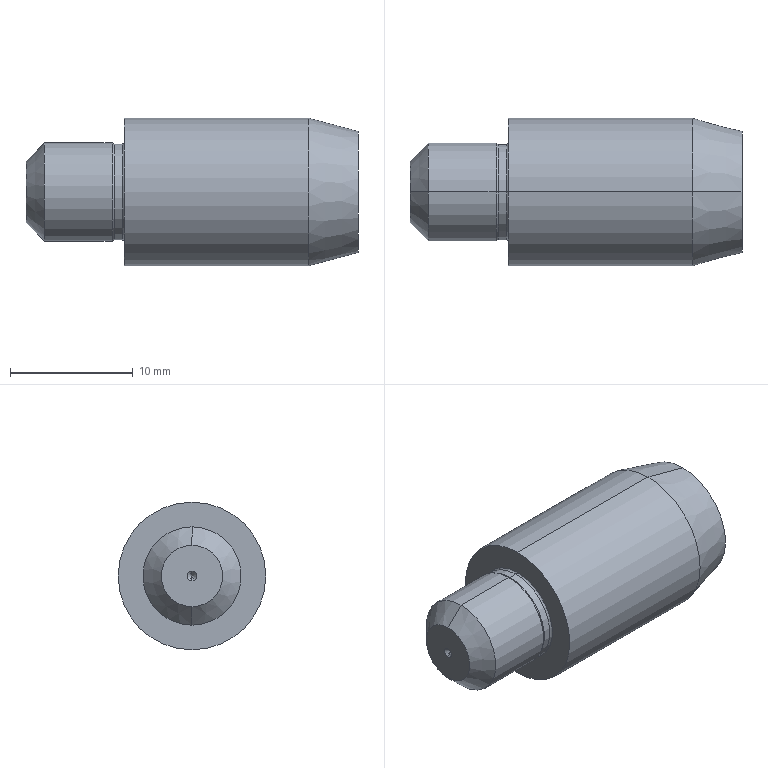Part | STEP file | FPBA8_P12_L9_B15_FPBA8-P12-L8-B15 | 1 solid | 21 faces | box 27 x 12 x 12 mm | volume 2448 mm3 | cone 8 | cylinder 6 | torus 4 | plane 3 | commonest cylinder face diameters 7.8 x2 8 x2 12 x2
STEP:
#1=CARTESIAN_POINT('',(0.,0.,0.));
#2=DIRECTION('',(0.,0.,1.));
#3=DIRECTION('',(1.,0.,0.));
#4=AXIS2_PLACEMENT_3D('',#1,#2,#3);
#5=CARTESIAN_POINT('',(19.,0.,-0.4));
#6=VERTEX_POINT('',#5);
#7=CARTESIAN_POINT('',(19.,0.,0.4));
#8=VERTEX_POINT('',#7);
#9=CARTESIAN_POINT('',(19.,0.,0.));
#10=DIRECTION('',(-1.,0.,0.));
#11=DIRECTION('',(0.,0.,1.));
#12=AXIS2_PLACEMENT_3D('',#9,#10,#11);
#13=CIRCLE('',#12,0.4);
#14=CARTESIAN_POINT('',(1018.6,0.,0.));
#15=DIRECTION('',(1.,0.,0.));
#16=DIRECTION('',(0.,0.,-1.));
#17=AXIS2_PLACEMENT_3D('',#14,#15,#16);
#18=CONICAL_SURFACE('',#17,1000.,0.7854);
#19=CARTESIAN_POINT('',(9.425,-999.6));
#20=DIRECTION('',(-1.,0.));
#21=VECTOR('',#20,1.);
#22=LINE('',#19,#21);
#23=(GEOMETRIC_REPRESENTATION_CONTEXT(2)PARAMETRIC_REPRESENTATION_CONTEXT()REPRESENTATION_CONTEXT('',''));
#24=DEFINITIONAL_REPRESENTATION('',(#22),#23);
#25=PCURVE('',#18,#24);
#26=CARTESIAN_POINT('',(19.,4.928,0.));
#27=DIRECTION('',(-1.,0.,0.));
#28=DIRECTION('',(0.,0.,1.));
#29=AXIS2_PLACEMENT_3D('',#26,#27,#28);
#30=PLANE('',#29);
#31=CARTESIAN_POINT('',(0.,-4.928));
#32=DIRECTION('',(1.,0.));
#33=AXIS2_PLACEMENT_2D('',#31,#32);
#34=CIRCLE('',#33,0.4);
#35=(GEOMETRIC_REPRESENTATION_CONTEXT(2)PARAMETRIC_REPRESENTATION_CONTEXT()REPRESENTATION_CONTEXT('',''));
#36=DEFINITIONAL_REPRESENTATION('',(#34),#35);
#37=PCURVE('',#30,#36);
#38=SURFACE_CURVE('',#13,(#25,#37),.PCURVE_S1.);
#39=EDGE_CURVE('',#6,#8,#38,.T.);
#40=ORIENTED_EDGE('',*,*,#39,.T.);
#41=CARTESIAN_POINT('',(18.6,0.,0.));
#42=VERTEX_POINT('',#41);
#43=CARTESIAN_POINT('',(18.6,0.,0.));
#44=DIRECTION('',(0.7071,0.,0.7071));
#45=VECTOR('',#44,1.);
#46=LINE('',#43,#45);
#47=CARTESIAN_POINT('',(3.142,-1000.));
#48=CARTESIAN_POINT('',(3.142,-999.994));
#49=CARTESIAN_POINT('',(3.142,-999.982));
#50=CARTESIAN_POINT('',(3.142,-999.964));
#51=CARTESIAN_POINT('',(3.142,-999.945));
#52=CARTESIAN_POINT('',(3.142,-999.927));
#53=CARTESIAN_POINT('',(3.142,-999.909));
#54=CARTESIAN_POINT('',(3.142,-999.891));
#55=CARTESIAN_POINT('',(3.142,-999.873));
#56=CARTESIAN_POINT('',(3.142,-999.855));
#57=CARTESIAN_POINT('',(3.142,-999.836));
#58=CARTESIAN_POINT('',(3.142,-999.818));
#59=CARTESIAN_POINT('',(3.142,-999.8));
#60=CARTESIAN_POINT('',(3.142,-999.782));
#61=CARTESIAN_POINT('',(3.142,-999.764));
#62=CARTESIAN_POINT('',(3.142,-999.745));
#63=CARTESIAN_POINT('',(3.142,-999.727));
#64=CARTESIAN_POINT('',(3.142,-999.709));
#65=CARTESIAN_POINT('',(3.142,-999.691));
#66=CARTESIAN_POINT('',(3.142,-999.673));
#67=CARTESIAN_POINT('',(3.142,-999.655));
#68=CARTESIAN_POINT('',(3.142,-999.636));
#69=CARTESIAN_POINT('',(3.142,-999.618));
#70=CARTESIAN_POINT('',(3.142,-999.606));
#71=CARTESIAN_POINT('',(3.142,-999.6));
#72=B_SPLINE_CURVE_WITH_KNOTS('',3,(#47,#48,#49,#50,#51,#52,#53,#54,#55,#56,#57,#58,#59,#60,#61,#62,#63,#64,#65,#66,#67,#68,#69,#70,#71),.UNSPECIFIED.,.F.,.F.,(4,1,1,1,1,1,1,1,1,1,1,1,1,1,1,1,1,1,1,1,1,1,4),(0.,0.02571,0.05143,0.07714,0.1029,0.1286,0.1543,0.18,0.2057,0.2314,0.2571,0.2828,0.3086,0.3343,0.36,0.3857,0.4114,0.4371,0.4628,0.4885,0.5143,0.54,0.5657),.QUASI_UNIFORM_KNOTS.);
#73=(GEOMETRIC_REPRESENTATION_CONTEXT(2)PARAMETRIC_REPRESENTATION_CONTEXT()REPRESENTATION_CONTEXT('',''));
#74=DEFINITIONAL_REPRESENTATION('',(#72),#73);
#75=PCURVE('',#18,#74);
#76=CARTESIAN_POINT('',(1018.6,0.,0.));
#77=DIRECTION('',(1.,0.,0.));
#78=DIRECTION('',(0.,0.,-1.));
#79=AXIS2_PLACEMENT_3D('',#76,#77,#78);
#80=CONICAL_SURFACE('',#79,1000.,0.7854);
#81=CARTESIAN_POINT('',(3.142,-1000.));
#82=CARTESIAN_POINT('',(3.142,-999.994));
#83=CARTESIAN_POINT('',(3.142,-999.982));
#84=CARTESIAN_POINT('',(3.142,-999.964));
#85=CARTESIAN_POINT('',(3.142,-999.945));
#86=CARTESIAN_POINT('',(3.142,-999.927));
#87=CARTESIAN_POINT('',(3.142,-999.909));
#88=CARTESIAN_POINT('',(3.142,-999.891));
#89=CARTESIAN_POINT('',(3.142,-999.873));
#90=CARTESIAN_POINT('',(3.142,-999.855));
#91=CARTESIAN_POINT('',(3.142,-999.836));
#92=CARTESIAN_POINT('',(3.142,-999.818));
#93=CARTESIAN_POINT('',(3.142,-999.8));
#94=CARTESIAN_POINT('',(3.142,-999.782));
#95=CARTESIAN_POINT('',(3.142,-999.764));
#96=CARTESIAN_POINT('',(3.142,-999.745));
#97=CARTESIAN_POINT('',(3.142,-999.727));
#98=CARTESIAN_POINT('',(3.142,-999.709));
#99=CARTESIAN_POINT('',(3.142,-999.691));
#100=CARTESIAN_POINT('',(3.142,-999.673));
#101=CARTESIAN_POINT('',(3.142,-999.655));
#102=CARTESIAN_POINT('',(3.142,-999.636));
#103=CARTESIAN_POINT('',(3.142,-999.618));
#104=CARTESIAN_POINT('',(3.142,-999.606));
#105=CARTESIAN_POINT('',(3.142,-999.6));
#106=B_SPLINE_CURVE_WITH_KNOTS('',3,(#81,#82,#83,#84,#85,#86,#87,#88,#89,#90,#91,#92,#93,#94,#95,#96,#97,#98,#99,#100,#101,#102,#103,#104,#105),.UNSPECIFIED.,.F.,.F.,(4,1,1,1,1,1,1,1,1,1,1,1,1,1,1,1,1,1,1,1,1,1,4),(0.,0.02571,0.05143,0.07714,0.1029,0.1286,0.1543,0.18,0.2057,0.2314,0.2571,0.2828,0.3086,0.3343,0.36,0.3857,0.4114,0.4371,0.4628,0.4885,0.5143,0.54,0.5657),.QUASI_UNIFORM_KNOTS.);
#107=(GEOMETRIC_REPRESENTATION_CONTEXT(2)PARAMETRIC_REPRESENTATION_CONTEXT()REPRESENTATION_CONTEXT('',''));
#108=DEFINITIONAL_REPRESENTATION('',(#106),#107);
#109=PCURVE('',#80,#108);
#110=SURFACE_CURVE('',#46,(#75,#109),.PCURVE_S1.);
#111=EDGE_CURVE('',#42,#8,#110,.T.);
#112=ORIENTED_EDGE('',*,*,#111,.F.);
#113=CARTESIAN_POINT('',(18.6,0.,0.));
#114=DIRECTION('',(0.7071,0.,-0.7071));
#115=VECTOR('',#114,1.);
#116=LINE('',#113,#115);
#117=CARTESIAN_POINT('',(6.283,-1000.));
#118=DIRECTION('',(0.,1.));
#119=VECTOR('',#118,1.);
#120=LINE('',#117,#119);
#121=(GEOMETRIC_REPRESENTATION_CONTEXT(2)PARAMETRIC_REPRESENTATION_CONTEXT()REPRESENTATION_CONTEXT('',''));
#122=DEFINITIONAL_REPRESENTATION('',(#120),#121);
#123=PCURVE('',#18,#122);
#124=CARTESIAN_POINT('',(0.,-1000.));
#125=DIRECTION('',(0.,1.));
#126=VECTOR('',#125,1.);
#127=LINE('',#124,#126);
#128=(GEOMETRIC_REPRESENTATION_CONTEXT(2)PARAMETRIC_REPRESENTATION_CONTEXT()REPRESENTATION_CONTEXT('',''));
#129=DEFINITIONAL_REPRESENTATION('',(#127),#128);
#130=PCURVE('',#80,#129);
#131=SURFACE_CURVE('',#116,(#123,#130),.PCURVE_S1.);
#132=EDGE_CURVE('',#42,#6,#131,.T.);
#133=ORIENTED_EDGE('',*,*,#132,.T.);
#134=EDGE_LOOP('',(#40,#112,#133));
#135=FACE_BOUND('',#134,.F.);
#136=ADVANCED_FACE('',(#135),#18,.F.);
#137=CARTESIAN_POINT('',(19.,0.,4.928));
#138=VERTEX_POINT('',#137);
#139=CARTESIAN_POINT('',(19.,0.,-4.928));
#140=VERTEX_POINT('',#139);
#141=CARTESIAN_POINT('',(19.,0.,0.));
#142=DIRECTION('',(-1.,0.,0.));
#143=DIRECTION('',(0.,0.,1.));
#144=AXIS2_PLACEMENT_3D('',#141,#142,#143);
#145=CIRCLE('',#144,4.928);
#146=CARTESIAN_POINT('',(19.,0.,0.));
#147=DIRECTION('',(-1.,0.,0.));
#148=DIRECTION('',(0.,0.,1.));
#149=AXIS2_PLACEMENT_3D('',#146,#147,#148);
#150=CONICAL_SURFACE('',#149,4.928,0.2618);
#151=CARTESIAN_POINT('',(0.,0.));
#152=DIRECTION('',(1.,0.));
#153=VECTOR('',#152,1.);
#154=LINE('',#151,#153);
#155=(GEOMETRIC_REPRESENTATION_CONTEXT(2)PARAMETRIC_REPRESENTATION_CONTEXT()REPRESENTATION_CONTEXT('',''));
#156=DEFINITIONAL_REPRESENTATION('',(#154),#155);
#157=PCURVE('',#150,#156);
#158=CARTESIAN_POINT('',(0.,-4.928));
#159=DIRECTION('',(1.,0.));
#160=AXIS2_PLACEMENT_2D('',#158,#159);
#161=CIRCLE('',#160,4.928);
#162=(GEOMETRIC_REPRESENTATION_CONTEXT(2)PARAMETRIC_REPRESENTATION_CONTEXT()REPRESENTATION_CONTEXT('',''));
#163=DEFINITIONAL_REPRESENTATION('',(#161),#162);
#164=PCURVE('',#30,#163);
#165=SURFACE_CURVE('',#145,(#157,#164),.PCURVE_S1.);
#166=EDGE_CURVE('',#138,#140,#165,.T.);
#167=ORIENTED_EDGE('',*,*,#166,.T.);
#168=CARTESIAN_POINT('',(15.,0.,-6.));
#169=VERTEX_POINT('',#168);
#170=CARTESIAN_POINT('',(19.,0.,-4.928));
#171=DIRECTION('',(-0.9659,0.,-0.2588));
#172=VECTOR('',#171,1.);
#173=LINE('',#170,#172);
#174=CARTESIAN_POINT('',(3.142,0.));
#175=DIRECTION('',(0.,1.));
#176=VECTOR('',#175,1.);
#177=LINE('',#174,#176);
#178=(GEOMETRIC_REPRESENTATION_CONTEXT(2)PARAMETRIC_REPRESENTATION_CONTEXT()REPRESENTATION_CONTEXT('',''));
#179=DEFINITIONAL_REPRESENTATION('',(#177),#178);
#180=PCURVE('',#150,#179);
#181=CARTESIAN_POINT('',(19.,0.,0.));
#182=DIRECTION('',(-1.,0.,0.));
#183=DIRECTION('',(0.,0.,1.));
#184=AXIS2_PLACEMENT_3D('',#181,#182,#183);
#185=CONICAL_SURFACE('',#184,4.928,0.2618);
#186=CARTESIAN_POINT('',(3.142,0.));
#187=DIRECTION('',(0.,1.));
#188=VECTOR('',#187,1.);
#189=LINE('',#186,#188);
#190=(GEOMETRIC_REPRESENTATION_CONTEXT(2)PARAMETRIC_REPRESENTATION_CONTEXT()REPRESENTATION_CONTEXT('',''));
#191=DEFINITIONAL_REPRESENTATION('',(#189),#190);
#192=PCURVE('',#185,#191);
#193=SURFACE_CURVE('',#173,(#180,#192),.PCURVE_S1.);
#194=EDGE_CURVE('',#140,#169,#193,.T.);
#195=ORIENTED_EDGE('',*,*,#194,.T.);
#196=CARTESIAN_POINT('',(15.,0.,6.));
#197=VERTEX_POINT('',#196);
#198=CARTESIAN_POINT('',(15.,0.,0.));
#199=DIRECTION('',(-1.,0.,0.));
#200=DIRECTION('',(0.,0.,1.));
#201=AXIS2_PLACEMENT_3D('',#198,#199,#200);
#202=CIRCLE('',#201,6.);
#203=CARTESIAN_POINT('',(0.,4.));
#204=DIRECTION('',(1.,0.));
#205=VECTOR('',#204,1.);
#206=LINE('',#203,#205);
#207=(GEOMETRIC_REPRESENTATION_CONTEXT(2)PARAMETRIC_REPRESENTATION_CONTEXT()REPRESENTATION_CONTEXT('',''));
#208=DEFINITIONAL_REPRESENTATION('',(#206),#207);
#209=PCURVE('',#150,#208);
#210=CARTESIAN_POINT('',(18.6,0.,0.));
#211=DIRECTION('',(-1.,0.,0.));
#212=DIRECTION('',(0.,0.,1.));
#213=AXIS2_PLACEMENT_3D('',#210,#211,#212);
#214=CYLINDRICAL_SURFACE('',#213,6.);
#215=CARTESIAN_POINT('',(0.,3.6));
#216=DIRECTION('',(1.,0.));
#217=VECTOR('',#216,1.);
#218=LINE('',#215,#217);
#219=(GEOMETRIC_REPRESENTATION_CONTEXT(2)PARAMETRIC_REPRESENTATION_CONTEXT()REPRESENTATION_CONTEXT('',''));
#220=DEFINITIONAL_REPRESENTATION('',(#218),#219);
#221=PCURVE('',#214,#220);
#222=SURFACE_CURVE('',#202,(#209,#221),.PCURVE_S1.);
#223=EDGE_CURVE('',#197,#169,#222,.T.);
#224=ORIENTED_EDGE('',*,*,#223,.F.);
#225=CARTESIAN_POINT('',(19.,0.,4.928));
#226=DIRECTION('',(-0.9659,0.,0.2588));
#227=VECTOR('',#226,1.);
#228=LINE('',#225,#227);
#229=CARTESIAN_POINT('',(0.,0.));
#230=DIRECTION('',(0.,1.));
#231=VECTOR('',#230,1.);
#232=LINE('',#229,#231);
#233=(GEOMETRIC_REPRESENTATION_CONTEXT(2)PARAMETRIC_REPRESENTATION_CONTEXT()REPRESENTATION_CONTEXT('',''));
#234=DEFINITIONAL_REPRESENTATION('',(#232),#233);
#235=PCURVE('',#150,#234);
#236=CARTESIAN_POINT('',(6.283,0.));
#237=DIRECTION('',(0.,1.));
#238=VECTOR('',#237,1.);
#239=LINE('',#236,#238);
#240=(GEOMETRIC_REPRESENTATION_CONTEXT(2)PARAMETRIC_REPRESENTATION_CONTEXT()REPRESENTATION_CONTEXT('',''));
#241=DEFINITIONAL_REPRESENTATION('',(#239),#240);
#242=PCURVE('',#185,#241);
#243=SURFACE_CURVE('',#228,(#235,#242),.PCURVE_S1.);
#244=EDGE_CURVE('',#138,#197,#243,.T.);
#245=ORIENTED_EDGE('',*,*,#244,.F.);
#246=EDGE_LOOP('',(#167,#195,#224,#245));
#247=FACE_BOUND('',#246,.T.);
#248=ADVANCED_FACE('',(#247),#150,.T.);
#249=ORIENTED_EDGE('',*,*,#223,.T.);
#250=CARTESIAN_POINT('',(0.,0.,-6.));
#251=VERTEX_POINT('',#250);
#252=CARTESIAN_POINT('',(18.6,0.,-6.));
#253=DIRECTION('',(-1.,0.,0.));
#254=VECTOR('',#253,1.);
#255=LINE('',#252,#254);
#256=CARTESIAN_POINT('',(3.142,0.));
#257=DIRECTION('',(0.,1.));
#258=VECTOR('',#257,1.);
#259=LINE('',#256,#258);
#260=(GEOMETRIC_REPRESENTATION_CONTEXT(2)PARAMETRIC_REPRESENTATION_CONTEXT()REPRESENTATION_CONTEXT('',''));
#261=DEFINITIONAL_REPRESENTATION('',(#259),#260);
#262=PCURVE('',#214,#261);
#263=CARTESIAN_POINT('',(18.6,0.,0.));
#264=DIRECTION('',(-1.,0.,0.));
#265=DIRECTION('',(0.,0.,1.));
#266=AXIS2_PLACEMENT_3D('',#263,#264,#265);
#267=CYLINDRICAL_SURFACE('',#266,6.);
#268=CARTESIAN_POINT('',(3.142,0.));
#269=DIRECTION('',(0.,1.));
#270=VECTOR('',#269,1.);
#271=LINE('',#268,#270);
#272=(GEOMETRIC_REPRESENTATION_CONTEXT(2)PARAMETRIC_REPRESENTATION_CONTEXT()REPRESENTATION_CONTEXT('',''));
#273=DEFINITIONAL_REPRESENTATION('',(#271),#272);
#274=PCURVE('',#267,#273);
#275=SURFACE_CURVE('',#255,(#262,#274),.PCURVE_S1.);
#276=EDGE_CURVE('',#169,#251,#275,.T.);
#277=ORIENTED_EDGE('',*,*,#276,.T.);
#278=CARTESIAN_POINT('',(0.,0.,6.));
#279=VERTEX_POINT('',#278);
#280=CARTESIAN_POINT('',(0.,0.,0.));
#281=DIRECTION('',(-1.,0.,0.));
#282=DIRECTION('',(0.,0.,1.));
#283=AXIS2_PLACEMENT_3D('',#280,#281,#282);
#284=CIRCLE('',#283,6.);
#285=CARTESIAN_POINT('',(0.,18.6));
#286=DIRECTION('',(1.,0.));
#287=VECTOR('',#286,1.);
#288=LINE('',#285,#287);
#289=(GEOMETRIC_REPRESENTATION_CONTEXT(2)PARAMETRIC_REPRESENTATION_CONTEXT()REPRESENTATION_CONTEXT('',''));
#290=DEFINITIONAL_REPRESENTATION('',(#288),#289);
#291=PCURVE('',#214,#290);
#292=CARTESIAN_POINT('',(0.,0.,0.));
#293=DIRECTION('',(1.,0.,0.));
#294=DIRECTION('',(0.,0.,-1.));
#295=AXIS2_PLACEMENT_3D('',#292,#293,#294);
#296=PLANE('',#295);
#297=CARTESIAN_POINT('',(-6.,0.));
#298=CARTESIAN_POINT('',(-6.,10.392));
#299=CARTESIAN_POINT('',(3.,5.196));
#300=CARTESIAN_POINT('',(12.,0.));
#301=CARTESIAN_POINT('',(3.,-5.196));
#302=CARTESIAN_POINT('',(-6.,-10.392));
#303=CARTESIAN_POINT('',(-6.,0.));
#304=(BOUNDED_CURVE()B_SPLINE_CURVE(2,(#297,#298,#299,#300,#301,#302,#303),.UNSPECIFIED.,.T.,.F.)B_SPLINE_CURVE_WITH_KNOTS((1,2,2,2,2,1),(-2.094,0.,2.094,4.189,6.283,8.378),.UNSPECIFIED.)CURVE()GEOMETRIC_REPRESENTATION_ITEM()RATIONAL_B_SPLINE_CURVE((1.,0.5,1.,0.5,1.,0.5,1.))REPRESENTATION_ITEM(''));
#305=(GEOMETRIC_REPRESENTATION_CONTEXT(2)PARAMETRIC_REPRESENTATION_CONTEXT()REPRESENTATION_CONTEXT('',''));
#306=DEFINITIONAL_REPRESENTATION('',(#304),#305);
#307=PCURVE('',#296,#306);
#308=SURFACE_CURVE('',#284,(#291,#307),.PCURVE_S1.);
#309=EDGE_CURVE('',#279,#251,#308,.T.);
#310=ORIENTED_EDGE('',*,*,#309,.F.);
#311=CARTESIAN_POINT('',(18.6,0.,6.));
#312=DIRECTION('',(-1.,0.,0.));
#313=VECTOR('',#312,1.);
#314=LINE('',#311,#313);
#315=CARTESIAN_POINT('',(0.,0.));
#316=DIRECTION('',(0.,1.));
#317=VECTOR('',#316,1.);
#318=LINE('',#315,#317);
#319=(GEOMETRIC_REPRESENTATION_CONTEXT(2)PARAMETRIC_REPRESENTATION_CONTEXT()REPRESENTATION_CONTEXT('',''));
#320=DEFINITIONAL_REPRESENTATION('',(#318),#319);
#321=PCURVE('',#214,#320);
#322=CARTESIAN_POINT('',(6.283,0.));
#323=DIRECTION('',(0.,1.));
#324=VECTOR('',#323,1.);
#325=LINE('',#322,#324);
#326=(GEOMETRIC_REPRESENTATION_CONTEXT(2)PARAMETRIC_REPRESENTATION_CONTEXT()REPRESENTATION_CONTEXT('',''));
#327=DEFINITIONAL_REPRESENTATION('',(#325),#326);
#328=PCURVE('',#267,#327);
#329=SURFACE_CURVE('',#314,(#321,#328),.PCURVE_S1.);
#330=EDGE_CURVE('',#197,#279,#329,.T.);
#331=ORIENTED_EDGE('',*,*,#330,.F.);
#332=EDGE_LOOP('',(#249,#277,#310,#331));
#333=FACE_BOUND('',#332,.T.);
#334=ADVANCED_FACE('',(#333),#214,.T.);
#335=CARTESIAN_POINT('',(-8.,0.,-0.4));
#336=VERTEX_POINT('',#335);
#337=CARTESIAN_POINT('',(-8.,0.,0.4));
#338=VERTEX_POINT('',#337);
#339=CARTESIAN_POINT('',(-8.,0.,0.));
#340=DIRECTION('',(-1.,0.,0.));
#341=DIRECTION('',(0.,0.,1.));
#342=AXIS2_PLACEMENT_3D('',#339,#340,#341);
#343=CIRCLE('',#342,0.4);
#344=CARTESIAN_POINT('',(-8.,0.,0.));
#345=DIRECTION('',(-1.,0.,0.));
#346=DIRECTION('',(0.,0.,1.));
#347=AXIS2_PLACEMENT_3D('',#344,#345,#346);
#348=CONICAL_SURFACE('',#347,0.4,0.7854);
#349=CARTESIAN_POINT('',(0.,0.));
#350=DIRECTION('',(1.,0.));
#351=VECTOR('',#350,1.);
#352=LINE('',#349,#351);
#353=(GEOMETRIC_REPRESENTATION_CONTEXT(2)PARAMETRIC_REPRESENTATION_CONTEXT()REPRESENTATION_CONTEXT('',''));
#354=DEFINITIONAL_REPRESENTATION('',(#352),#353);
#355=PCURVE('',#348,#354);
#356=CARTESIAN_POINT('',(-8.,0.4,0.));
#357=DIRECTION('',(1.,0.,0.));
#358=DIRECTION('',(0.,0.,-1.));
#359=AXIS2_PLACEMENT_3D('',#356,#357,#358);
#360=PLANE('',#359);
#361=CARTESIAN_POINT('',(-0.4,-0.4));
#362=CARTESIAN_POINT('',(-0.4,0.2928));
#363=CARTESIAN_POINT('',(0.2,-0.05359));
#364=CARTESIAN_POINT('',(0.8,-0.4));
#365=CARTESIAN_POINT('',(0.2,-0.7464));
#366=CARTESIAN_POINT('',(-0.4,-1.093));
#367=CARTESIAN_POINT('',(-0.4,-0.4));
#368=(BOUNDED_CURVE()B_SPLINE_CURVE(2,(#361,#362,#363,#364,#365,#366,#367),.UNSPECIFIED.,.T.,.F.)B_SPLINE_CURVE_WITH_KNOTS((1,2,2,2,2,1),(-2.094,0.,2.094,4.189,6.283,8.378),.UNSPECIFIED.)CURVE()GEOMETRIC_REPRESENTATION_ITEM()RATIONAL_B_SPLINE_CURVE((1.,0.5,1.,0.5,1.,0.5,1.))REPRESENTATION_ITEM(''));
#369=(GEOMETRIC_REPRESENTATION_CONTEXT(2)PARAMETRIC_REPRESENTATION_CONTEXT()REPRESENTATION_CONTEXT('',''));
#370=DEFINITIONAL_REPRESENTATION('',(#368),#369);
#371=PCURVE('',#360,#370);
#372=SURFACE_CURVE('',#343,(#355,#371),.PCURVE_S1.);
#373=EDGE_CURVE('',#336,#338,#372,.T.);
#374=ORIENTED_EDGE('',*,*,#373,.F.);
#375=CARTESIAN_POINT('',(-7.6,0.,0.));
#376=VERTEX_POINT('',#375);
#377=CARTESIAN_POINT('',(-8.,0.,-0.4));
#378=DIRECTION('',(-0.7071,0.,-0.7071));
#379=VECTOR('',#378,1.);
#380=LINE('',#377,#379);
#381=CARTESIAN_POINT('',(3.142,0.));
#382=DIRECTION('',(0.,1.));
#383=VECTOR('',#382,1.);
#384=LINE('',#381,#383);
#385=(GEOMETRIC_REPRESENTATION_CONTEXT(2)PARAMETRIC_REPRESENTATION_CONTEXT()REPRESENTATION_CONTEXT('',''));
#386=DEFINITIONAL_REPRESENTATION('',(#384),#385);
#387=PCURVE('',#348,#386);
#388=CARTESIAN_POINT('',(-8.,0.,0.));
#389=DIRECTION('',(-1.,0.,0.));
#390=DIRECTION('',(0.,0.,1.));
#391=AXIS2_PLACEMENT_3D('',#388,#389,#390);
#392=CONICAL_SURFACE('',#391,0.4,0.7854);
#393=CARTESIAN_POINT('',(3.142,0.));
#394=DIRECTION('',(0.,1.));
#395=VECTOR('',#394,1.);
#396=LINE('',#393,#395);
#397=(GEOMETRIC_REPRESENTATION_CONTEXT(2)PARAMETRIC_REPRESENTATION_CONTEXT()REPRESENTATION_CONTEXT('',''));
#398=DEFINITIONAL_REPRESENTATION('',(#396),#397);
#399=PCURVE('',#392,#398);
#400=SURFACE_CURVE('',#380,(#387,#399),.PCURVE_S1.);
#401=EDGE_CURVE('',#376,#336,#400,.T.);
#402=ORIENTED_EDGE('',*,*,#401,.F.);
#403=CARTESIAN_POINT('',(-8.,0.,0.4));
#404=DIRECTION('',(-0.7071,0.,0.7071));
#405=VECTOR('',#404,1.);
#406=LINE('',#403,#405);
#407=CARTESIAN_POINT('',(6.283,0.));
#408=DIRECTION('',(0.,1.));
#409=VECTOR('',#408,1.);
#410=LINE('',#407,#409);
#411=(GEOMETRIC_REPRESENTATION_CONTEXT(2)PARAMETRIC_REPRESENTATION_CONTEXT()REPRESENTATION_CONTEXT('',''));
#412=DEFINITIONAL_REPRESENTATION('',(#410),#411);
#413=PCURVE('',#348,#412);
#414=CARTESIAN_POINT('',(0.,0.));
#415=DIRECTION('',(0.,1.));
#416=VECTOR('',#415,1.);
#417=LINE('',#414,#416);
#418=(GEOMETRIC_REPRESENTATION_CONTEXT(2)PARAMETRIC_REPRESENTATION_CONTEXT()REPRESENTATION_CONTEXT('',''));
#419=DEFINITIONAL_REPRESENTATION('',(#417),#418);
#420=PCURVE('',#392,#419);
#421=SURFACE_CURVE('',#406,(#413,#420),.PCURVE_S1.);
#422=EDGE_CURVE('',#376,#338,#421,.T.);
#423=ORIENTED_EDGE('',*,*,#422,.T.);
#424=EDGE_LOOP('',(#374,#402,#423));
#425=FACE_BOUND('',#424,.F.);
#426=ADVANCED_FACE('',(#425),#348,.F.);
#427=CARTESIAN_POINT('',(-8.,0.,2.5));
#428=VERTEX_POINT('',#427);
#429=CARTESIAN_POINT('',(-8.,0.,-2.5));
#430=VERTEX_POINT('',#429);
#431=CARTESIAN_POINT('',(-8.,0.,0.));
#432=DIRECTION('',(-1.,0.,0.));
#433=DIRECTION('',(0.,0.,1.));
#434=AXIS2_PLACEMENT_3D('',#431,#432,#433);
#435=CIRCLE('',#434,2.5);
#436=CARTESIAN_POINT('',(-6.5,0.,0.));
#437=DIRECTION('',(1.,0.,0.));
#438=DIRECTION('',(0.,0.,-1.));
#439=AXIS2_PLACEMENT_3D('',#436,#437,#438);
#440=CONICAL_SURFACE('',#439,4.,0.7854);
#441=CARTESIAN_POINT('',(3.142,-1.5));
#442=DIRECTION('',(-1.,0.));
#443=VECTOR('',#442,1.);
#444=LINE('',#441,#443);
#445=(GEOMETRIC_REPRESENTATION_CONTEXT(2)PARAMETRIC_REPRESENTATION_CONTEXT()REPRESENTATION_CONTEXT('',''));
#446=DEFINITIONAL_REPRESENTATION('',(#444),#445);
#447=PCURVE('',#440,#446);
#448=CARTESIAN_POINT('',(-2.5,-0.4));
#449=CARTESIAN_POINT('',(-2.5,3.93));
#450=CARTESIAN_POINT('',(1.25,1.765));
#451=CARTESIAN_POINT('',(5.,-0.4));
#452=CARTESIAN_POINT('',(1.25,-2.565));
#453=CARTESIAN_POINT('',(-2.5,-4.73));
#454=CARTESIAN_POINT('',(-2.5,-0.4));
#455=(BOUNDED_CURVE()B_SPLINE_CURVE(2,(#448,#449,#450,#451,#452,#453,#454),.UNSPECIFIED.,.T.,.F.)B_SPLINE_CURVE_WITH_KNOTS((1,2,2,2,2,1),(-2.094,0.,2.094,4.189,6.283,8.378),.UNSPECIFIED.)CURVE()GEOMETRIC_REPRESENTATION_ITEM()RATIONAL_B_SPLINE_CURVE((1.,0.5,1.,0.5,1.,0.5,1.))REPRESENTATION_ITEM(''));
#456=(GEOMETRIC_REPRESENTATION_CONTEXT(2)PARAMETRIC_REPRESENTATION_CONTEXT()REPRESENTATION_CONTEXT('',''));
#457=DEFINITIONAL_REPRESENTATION('',(#455),#456);
#458=PCURVE('',#360,#457);
#459=SURFACE_CURVE('',#435,(#447,#458),.PCURVE_S1.);
#460=EDGE_CURVE('',#428,#430,#459,.T.);
#461=ORIENTED_EDGE('',*,*,#460,.F.);
#462=CARTESIAN_POINT('',(-6.5,0.,4.));
#463=VERTEX_POINT('',#462);
#464=CARTESIAN_POINT('',(-6.5,0.,4.));
#465=DIRECTION('',(0.7071,0.,0.7071));
#466=VECTOR('',#465,1.);
#467=LINE('',#464,#466);
#468=CARTESIAN_POINT('',(3.142,0.));
#469=DIRECTION('',(0.,1.));
#470=VECTOR('',#469,1.);
#471=LINE('',#468,#470);
#472=(GEOMETRIC_REPRESENTATION_CONTEXT(2)PARAMETRIC_REPRESENTATION_CONTEXT()REPRESENTATION_CONTEXT('',''));
#473=DEFINITIONAL_REPRESENTATION('',(#471),#472);
#474=PCURVE('',#440,#473);
#475=CARTESIAN_POINT('',(-6.5,0.,0.));
#476=DIRECTION('',(1.,0.,0.));
#477=DIRECTION('',(0.,0.,-1.));
#478=AXIS2_PLACEMENT_3D('',#475,#476,#477);
#479=CONICAL_SURFACE('',#478,4.,0.7854);
#480=CARTESIAN_POINT('',(3.142,0.));
#481=DIRECTION('',(0.,1.));
#482=VECTOR('',#481,1.);
#483=LINE('',#480,#482);
#484=(GEOMETRIC_REPRESENTATION_CONTEXT(2)PARAMETRIC_REPRESENTATION_CONTEXT()REPRESENTATION_CONTEXT('',''));
#485=DEFINITIONAL_REPRESENTATION('',(#483),#484);
#486=PCURVE('',#479,#485);
#487=SURFACE_CURVE('',#467,(#474,#486),.PCURVE_S1.);
#488=EDGE_CURVE('',#428,#463,#487,.T.);
#489=ORIENTED_EDGE('',*,*,#488,.T.);
#490=CARTESIAN_POINT('',(-6.5,0.,-4.));
#491=VERTEX_POINT('',#490);
#492=CARTESIAN_POINT('',(-6.5,0.,0.));
#493=DIRECTION('',(-1.,0.,0.));
#494=DIRECTION('',(0.,0.,1.));
#495=AXIS2_PLACEMENT_3D('',#492,#493,#494);
#496=CIRCLE('',#495,4.);
#497=CARTESIAN_POINT('',(3.142,0.));
#498=DIRECTION('',(-1.,0.));
#499=VECTOR('',#498,1.);
#500=LINE('',#497,#499);
#501=(GEOMETRIC_REPRESENTATION_CONTEXT(2)PARAMETRIC_REPRESENTATION_CONTEXT()REPRESENTATION_CONTEXT('',''));
#502=DEFINITIONAL_REPRESENTATION('',(#500),#501);
#503=PCURVE('',#440,#502);
#504=CARTESIAN_POINT('',(0.,0.,0.));
#505=DIRECTION('',(-1.,0.,0.));
#506=DIRECTION('',(0.,0.,1.));
#507=AXIS2_PLACEMENT_3D('',#504,#505,#506);
#508=CYLINDRICAL_SURFACE('',#507,4.);
#509=CARTESIAN_POINT('',(0.,6.5));
#510=DIRECTION('',(1.,0.));
#511=VECTOR('',#510,1.);
#512=LINE('',#509,#511);
#513=(GEOMETRIC_REPRESENTATION_CONTEXT(2)PARAMETRIC_REPRESENTATION_CONTEXT()REPRESENTATION_CONTEXT('',''));
#514=DEFINITIONAL_REPRESENTATION('',(#512),#513);
#515=PCURVE('',#508,#514);
#516=SURFACE_CURVE('',#496,(#503,#515),.PCURVE_S1.);
#517=EDGE_CURVE('',#463,#491,#516,.T.);
#518=ORIENTED_EDGE('',*,*,#517,.T.);
#519=CARTESIAN_POINT('',(-6.5,0.,-4.));
#520=DIRECTION('',(0.7071,0.,-0.7071));
#521=VECTOR('',#520,1.);
#522=LINE('',#519,#521);
#523=CARTESIAN_POINT('',(0.,0.));
#524=DIRECTION('',(0.,1.));
#525=VECTOR('',#524,1.);
#526=LINE('',#523,#525);
#527=(GEOMETRIC_REPRESENTATION_CONTEXT(2)PARAMETRIC_REPRESENTATION_CONTEXT()REPRESENTATION_CONTEXT('',''));
#528=DEFINITIONAL_REPRESENTATION('',(#526),#527);
#529=PCURVE('',#440,#528);
#530=CARTESIAN_POINT('',(6.283,0.));
#531=DIRECTION('',(0.,1.));
#532=VECTOR('',#531,1.);
#533=LINE('',#530,#532);
#534=(GEOMETRIC_REPRESENTATION_CONTEXT(2)PARAMETRIC_REPRESENTATION_CONTEXT()REPRESENTATION_CONTEXT('',''));
#535=DEFINITIONAL_REPRESENTATION('',(#533),#534);
#536=PCURVE('',#479,#535);
#537=SURFACE_CURVE('',#522,(#529,#536),.PCURVE_S1.);
#538=EDGE_CURVE('',#430,#491,#537,.T.);
#539=ORIENTED_EDGE('',*,*,#538,.F.);
#540=EDGE_LOOP('',(#461,#489,#518,#539));
#541=FACE_BOUND('',#540,.T.);
#542=ADVANCED_FACE('',(#541),#440,.T.);
#543=CARTESIAN_POINT('',(-1.,0.,4.));
#544=VERTEX_POINT('',#543);
#545=CARTESIAN_POINT('',(-1.,0.,-4.));
#546=VERTEX_POINT('',#545);
#547=CARTESIAN_POINT('',(-1.,0.,0.));
#548=DIRECTION('',(-1.,0.,0.));
#549=DIRECTION('',(0.,0.,1.));
#550=AXIS2_PLACEMENT_3D('',#547,#548,#549);
#551=CIRCLE('',#550,4.);
#552=CARTESIAN_POINT('',(0.,1.));
#553=DIRECTION('',(1.,0.));
#554=VECTOR('',#553,1.);
#555=LINE('',#552,#554);
#556=(GEOMETRIC_REPRESENTATION_CONTEXT(2)PARAMETRIC_REPRESENTATION_CONTEXT()REPRESENTATION_CONTEXT('',''));
#557=DEFINITIONAL_REPRESENTATION('',(#555),#556);
#558=PCURVE('',#508,#557);
#559=CARTESIAN_POINT('',(-0.8268,0.,0.));
#560=DIRECTION('',(-1.,0.,0.));
#561=DIRECTION('',(0.,0.,1.));
#562=AXIS2_PLACEMENT_3D('',#559,#560,#561);
#563=TOROIDAL_SURFACE('',#562,4.1,0.2);
#564=CARTESIAN_POINT('',(0.,2.094));
#565=DIRECTION('',(1.,0.));
#566=VECTOR('',#565,1.);
#567=LINE('',#564,#566);
#568=(GEOMETRIC_REPRESENTATION_CONTEXT(2)PARAMETRIC_REPRESENTATION_CONTEXT()REPRESENTATION_CONTEXT('',''));
#569=DEFINITIONAL_REPRESENTATION('',(#567),#568);
#570=PCURVE('',#563,#569);
#571=SURFACE_CURVE('',#551,(#558,#570),.PCURVE_S1.);
#572=EDGE_CURVE('',#544,#546,#571,.T.);
#573=ORIENTED_EDGE('',*,*,#572,.T.);
#574=CARTESIAN_POINT('',(0.,0.,-4.));
#575=DIRECTION('',(-1.,0.,0.));
#576=VECTOR('',#575,1.);
#577=LINE('',#574,#576);
#578=CARTESIAN_POINT('',(3.142,0.));
#579=DIRECTION('',(0.,1.));
#580=VECTOR('',#579,1.);
#581=LINE('',#578,#580);
#582=(GEOMETRIC_REPRESENTATION_CONTEXT(2)PARAMETRIC_REPRESENTATION_CONTEXT()REPRESENTATION_CONTEXT('',''));
#583=DEFINITIONAL_REPRESENTATION('',(#581),#582);
#584=PCURVE('',#508,#583);
#585=CARTESIAN_POINT('',(0.,0.,0.));
#586=DIRECTION('',(-1.,0.,0.));
#587=DIRECTION('',(0.,0.,1.));
#588=AXIS2_PLACEMENT_3D('',#585,#586,#587);
#589=CYLINDRICAL_SURFACE('',#588,4.);
#590=CARTESIAN_POINT('',(3.142,0.));
#591=DIRECTION('',(0.,1.));
#592=VECTOR('',#591,1.);
#593=LINE('',#590,#592);
#594=(GEOMETRIC_REPRESENTATION_CONTEXT(2)PARAMETRIC_REPRESENTATION_CONTEXT()REPRESENTATION_CONTEXT('',''));
#595=DEFINITIONAL_REPRESENTATION('',(#593),#594);
#596=PCURVE('',#589,#595);
#597=SURFACE_CURVE('',#577,(#584,#596),.PCURVE_S1.);
#598=EDGE_CURVE('',#546,#491,#597,.T.);
#599=ORIENTED_EDGE('',*,*,#598,.T.);
#600=ORIENTED_EDGE('',*,*,#517,.F.);
#601=CARTESIAN_POINT('',(0.,0.,4.));
#602=DIRECTION('',(-1.,0.,0.));
#603=VECTOR('',#602,1.);
#604=LINE('',#601,#603);
#605=CARTESIAN_POINT('',(0.,0.));
#606=DIRECTION('',(0.,1.));
#607=VECTOR('',#606,1.);
#608=LINE('',#605,#607);
#609=(GEOMETRIC_REPRESENTATION_CONTEXT(2)PARAMETRIC_REPRESENTATION_CONTEXT()REPRESENTATION_CONTEXT('',''));
#610=DEFINITIONAL_REPRESENTATION('',(#608),#609);
#611=PCURVE('',#508,#610);
#612=CARTESIAN_POINT('',(6.283,0.));
#613=DIRECTION('',(0.,1.));
#614=VECTOR('',#613,1.);
#615=LINE('',#612,#614);
#616=(GEOMETRIC_REPRESENTATION_CONTEXT(2)PARAMETRIC_REPRESENTATION_CONTEXT()REPRESENTATION_CONTEXT('',''));
#617=DEFINITIONAL_REPRESENTATION('',(#615),#616);
#618=PCURVE('',#589,#617);
#619=SURFACE_CURVE('',#604,(#611,#618),.PCURVE_S1.);
#620=EDGE_CURVE('',#544,#463,#619,.T.);
#621=ORIENTED_EDGE('',*,*,#620,.F.);
#622=EDGE_LOOP('',(#573,#599,#600,#621));
#623=FACE_BOUND('',#622,.T.);
#624=ADVANCED_FACE('',(#623),#508,.T.);
#625=CARTESIAN_POINT('',(-0.8268,0.,3.9));
#626=VERTEX_POINT('',#625);
#627=CARTESIAN_POINT('',(-0.8268,0.,4.1));
#628=DIRECTION('',(0.,-1.,0.));
#629=DIRECTION('',(0.,0.,-1.));
#630=AXIS2_PLACEMENT_3D('',#627,#628,#629);
#631=CIRCLE('',#630,0.2);
#632=CARTESIAN_POINT('',(-0.8268,0.,0.));
#633=DIRECTION('',(-1.,0.,0.));
#634=DIRECTION('',(0.,0.,1.));
#635=AXIS2_PLACEMENT_3D('',#632,#633,#634);
#636=TOROIDAL_SURFACE('',#635,4.1,0.2);
#637=CARTESIAN_POINT('',(6.283,-3.142));
#638=DIRECTION('',(0.,1.));
#639=VECTOR('',#638,1.);
#640=LINE('',#637,#639);
#641=(GEOMETRIC_REPRESENTATION_CONTEXT(2)PARAMETRIC_REPRESENTATION_CONTEXT()REPRESENTATION_CONTEXT('',''));
#642=DEFINITIONAL_REPRESENTATION('',(#640),#641);
#643=PCURVE('',#636,#642);
#644=CARTESIAN_POINT('',(0.,-3.142));
#645=DIRECTION('',(0.,1.));
#646=VECTOR('',#645,1.);
#647=LINE('',#644,#646);
#648=(GEOMETRIC_REPRESENTATION_CONTEXT(2)PARAMETRIC_REPRESENTATION_CONTEXT()REPRESENTATION_CONTEXT('',''));
#649=DEFINITIONAL_REPRESENTATION('',(#647),#648);
#650=PCURVE('',#563,#649);
#651=SURFACE_CURVE('',#631,(#643,#650),.PCURVE_S1.);
#652=EDGE_CURVE('',#544,#626,#651,.T.);
#653=ORIENTED_EDGE('',*,*,#652,.T.);
#654=CARTESIAN_POINT('',(-0.8268,0.,-3.9));
#655=VERTEX_POINT('',#654);
#656=CARTESIAN_POINT('',(-0.8268,0.,0.));
#657=DIRECTION('',(-1.,0.,0.));
#658=DIRECTION('',(0.,0.,1.));
#659=AXIS2_PLACEMENT_3D('',#656,#657,#658);
#660=CIRCLE('',#659,3.9);
#661=CARTESIAN_POINT('',(0.,3.142));
#662=DIRECTION('',(1.,0.));
#663=VECTOR('',#662,1.);
#664=LINE('',#661,#663);
#665=(GEOMETRIC_REPRESENTATION_CONTEXT(2)PARAMETRIC_REPRESENTATION_CONTEXT()REPRESENTATION_CONTEXT('',''));
#666=DEFINITIONAL_REPRESENTATION('',(#664),#665);
#667=PCURVE('',#636,#666);
#668=CARTESIAN_POINT('',(0.,0.,0.));
#669=DIRECTION('',(-1.,0.,0.));
#670=DIRECTION('',(0.,0.,1.));
#671=AXIS2_PLACEMENT_3D('',#668,#669,#670);
#672=CYLINDRICAL_SURFACE('',#671,3.9);
#673=CARTESIAN_POINT('',(0.,0.8268));
#674=DIRECTION('',(1.,0.));
#675=VECTOR('',#674,1.);
#676=LINE('',#673,#675);
#677=(GEOMETRIC_REPRESENTATION_CONTEXT(2)PARAMETRIC_REPRESENTATION_CONTEXT()REPRESENTATION_CONTEXT('',''));
#678=DEFINITIONAL_REPRESENTATION('',(#676),#677);
#679=PCURVE('',#672,#678);
#680=SURFACE_CURVE('',#660,(#667,#679),.PCURVE_S1.);
#681=EDGE_CURVE('',#655,#626,#680,.T.);
#682=ORIENTED_EDGE('',*,*,#681,.F.);
#683=CARTESIAN_POINT('',(-0.8268,0.,-4.1));
#684=DIRECTION('',(0.,1.,0.));
#685=DIRECTION('',(0.,0.,1.));
#686=AXIS2_PLACEMENT_3D('',#683,#684,#685);
#687=CIRCLE('',#686,0.2);
#688=CARTESIAN_POINT('',(3.142,-3.142));
#689=DIRECTION('',(0.,1.));
#690=VECTOR('',#689,1.);
#691=LINE('',#688,#690);
#692=(GEOMETRIC_REPRESENTATION_CONTEXT(2)PARAMETRIC_REPRESENTATION_CONTEXT()REPRESENTATION_CONTEXT('',''));
#693=DEFINITIONAL_REPRESENTATION('',(#691),#692);
#694=PCURVE('',#636,#693);
#695=CARTESIAN_POINT('',(3.142,-3.142));
#696=DIRECTION('',(0.,1.));
#697=VECTOR('',#696,1.);
#698=LINE('',#695,#697);
#699=(GEOMETRIC_REPRESENTATION_CONTEXT(2)PARAMETRIC_REPRESENTATION_CONTEXT()REPRESENTATION_CONTEXT('',''));
#700=DEFINITIONAL_REPRESENTATION('',(#698),#699);
#701=PCURVE('',#563,#700);
#702=SURFACE_CURVE('',#687,(#694,#701),.PCURVE_S1.);
#703=EDGE_CURVE('',#546,#655,#702,.T.);
#704=ORIENTED_EDGE('',*,*,#703,.F.);
#705=CARTESIAN_POINT('',(-1.,0.,0.));
#706=DIRECTION('',(-1.,0.,0.));
#707=DIRECTION('',(0.,0.,1.));
#708=AXIS2_PLACEMENT_3D('',#705,#706,#707);
#709=CIRCLE('',#708,4.);
#710=CARTESIAN_POINT('',(0.,2.094));
#711=DIRECTION('',(1.,0.));
#712=VECTOR('',#711,1.);
#713=LINE('',#710,#712);
#714=(GEOMETRIC_REPRESENTATION_CONTEXT(2)PARAMETRIC_REPRESENTATION_CONTEXT()REPRESENTATION_CONTEXT('',''));
#715=DEFINITIONAL_REPRESENTATION('',(#713),#714);
#716=PCURVE('',#636,#715);
#717=CARTESIAN_POINT('',(0.,1.));
#718=DIRECTION('',(1.,0.));
#719=VECTOR('',#718,1.);
#720=LINE('',#717,#719);
#721=(GEOMETRIC_REPRESENTATION_CONTEXT(2)PARAMETRIC_REPRESENTATION_CONTEXT()REPRESENTATION_CONTEXT('',''));
#722=DEFINITIONAL_REPRESENTATION('',(#720),#721);
#723=PCURVE('',#589,#722);
#724=SURFACE_CURVE('',#709,(#716,#723),.PCURVE_S1.);
#725=EDGE_CURVE('',#546,#544,#724,.T.);
#726=ORIENTED_EDGE('',*,*,#725,.T.);
#727=EDGE_LOOP('',(#653,#682,#704,#726));
#728=FACE_BOUND('',#727,.F.);
#729=ADVANCED_FACE('',(#728),#636,.F.);
#730=CARTESIAN_POINT('',(-0.1732,0.,3.9));
#731=VERTEX_POINT('',#730);
#732=CARTESIAN_POINT('',(-0.1732,0.,-3.9));
#733=VERTEX_POINT('',#732);
#734=CARTESIAN_POINT('',(-0.1732,0.,0.));
#735=DIRECTION('',(-1.,0.,0.));
#736=DIRECTION('',(0.,0.,1.));
#737=AXIS2_PLACEMENT_3D('',#734,#735,#736);
#738=CIRCLE('',#737,3.9);
#739=CARTESIAN_POINT('',(0.,0.,0.));
#740=DIRECTION('',(-1.,0.,0.));
#741=DIRECTION('',(0.,0.,1.));
#742=AXIS2_PLACEMENT_3D('',#739,#740,#741);
#743=CYLINDRICAL_SURFACE('',#742,3.9);
#744=CARTESIAN_POINT('',(0.,0.1732));
#745=DIRECTION('',(1.,0.));
#746=VECTOR('',#745,1.);
#747=LINE('',#744,#746);
#748=(GEOMETRIC_REPRESENTATION_CONTEXT(2)PARAMETRIC_REPRESENTATION_CONTEXT()REPRESENTATION_CONTEXT('',''));
#749=DEFINITIONAL_REPRESENTATION('',(#747),#748);
#750=PCURVE('',#743,#749);
#751=CARTESIAN_POINT('',(-0.1732,0.,0.));
#752=DIRECTION('',(-1.,0.,0.));
#753=DIRECTION('',(0.,0.,1.));
#754=AXIS2_PLACEMENT_3D('',#751,#752,#753);
#755=TOROIDAL_SURFACE('',#754,4.1,0.2);
#756=CARTESIAN_POINT('',(0.,3.142));
#757=DIRECTION('',(1.,0.));
#758=VECTOR('',#757,1.);
#759=LINE('',#756,#758);
#760=(GEOMETRIC_REPRESENTATION_CONTEXT(2)PARAMETRIC_REPRESENTATION_CONTEXT()REPRESENTATION_CONTEXT('',''));
#761=DEFINITIONAL_REPRESENTATION('',(#759),#760);
#762=PCURVE('',#755,#761);
#763=SURFACE_CURVE('',#738,(#750,#762),.PCURVE_S1.);
#764=EDGE_CURVE('',#731,#733,#763,.T.);
#765=ORIENTED_EDGE('',*,*,#764,.T.);
#766=CARTESIAN_POINT('',(0.,0.,-3.9));
#767=DIRECTION('',(-1.,0.,0.));
#768=VECTOR('',#767,1.);
#769=LINE('',#766,#768);
#770=CARTESIAN_POINT('',(3.142,0.));
#771=DIRECTION('',(0.,1.));
#772=VECTOR('',#771,1.);
#773=LINE('',#770,#772);
#774=(GEOMETRIC_REPRESENTATION_CONTEXT(2)PARAMETRIC_REPRESENTATION_CONTEXT()REPRESENTATION_CONTEXT('',''));
#775=DEFINITIONAL_REPRESENTATION('',(#773),#774);
#776=PCURVE('',#743,#775);
#777=CARTESIAN_POINT('',(3.142,0.));
#778=DIRECTION('',(0.,1.));
#779=VECTOR('',#778,1.);
#780=LINE('',#777,#779);
#781=(GEOMETRIC_REPRESENTATION_CONTEXT(2)PARAMETRIC_REPRESENTATION_CONTEXT()REPRESENTATION_CONTEXT('',''));
#782=DEFINITIONAL_REPRESENTATION('',(#780),#781);
#783=PCURVE('',#672,#782);
#784=SURFACE_CURVE('',#769,(#776,#783),.PCURVE_S1.);
#785=EDGE_CURVE('',#733,#655,#784,.T.);
#786=ORIENTED_EDGE('',*,*,#785,.T.);
#787=CARTESIAN_POINT('',(-0.8268,0.,0.));
#788=DIRECTION('',(-1.,0.,0.));
#789=DIRECTION('',(0.,0.,1.));
#790=AXIS2_PLACEMENT_3D('',#787,#788,#789);
#791=CIRCLE('',#790,3.9);
#792=CARTESIAN_POINT('',(0.,0.8268));
#793=DIRECTION('',(1.,0.));
#794=VECTOR('',#793,1.);
#795=LINE('',#792,#794);
#796=(GEOMETRIC_REPRESENTATION_CONTEXT(2)PARAMETRIC_REPRESENTATION_CONTEXT()REPRESENTATION_CONTEXT('',''));
#797=DEFINITIONAL_REPRESENTATION('',(#795),#796);
#798=PCURVE('',#743,#797);
#799=CARTESIAN_POINT('',(0.,3.142));
#800=DIRECTION('',(1.,0.));
#801=VECTOR('',#800,1.);
#802=LINE('',#799,#801);
#803=(GEOMETRIC_REPRESENTATION_CONTEXT(2)PARAMETRIC_REPRESENTATION_CONTEXT()REPRESENTATION_CONTEXT('',''));
#804=DEFINITIONAL_REPRESENTATION('',(#802),#803);
#805=PCURVE('',#563,#804);
#806=SURFACE_CURVE('',#791,(#798,#805),.PCURVE_S1.);
#807=EDGE_CURVE('',#626,#655,#806,.T.);
#808=ORIENTED_EDGE('',*,*,#807,.F.);
#809=CARTESIAN_POINT('',(0.,0.,3.9));
#810=DIRECTION('',(-1.,0.,0.));
#811=VECTOR('',#810,1.);
#812=LINE('',#809,#811);
#813=CARTESIAN_POINT('',(0.,0.));
#814=DIRECTION('',(0.,1.));
#815=VECTOR('',#814,1.);
#816=LINE('',#813,#815);
#817=(GEOMETRIC_REPRESENTATION_CONTEXT(2)PARAMETRIC_REPRESENTATION_CONTEXT()REPRESENTATION_CONTEXT('',''));
#818=DEFINITIONAL_REPRESENTATION('',(#816),#817);
#819=PCURVE('',#743,#818);
#820=CARTESIAN_POINT('',(6.283,0.));
#821=DIRECTION('',(0.,1.));
#822=VECTOR('',#821,1.);
#823=LINE('',#820,#822);
#824=(GEOMETRIC_REPRESENTATION_CONTEXT(2)PARAMETRIC_REPRESENTATION_CONTEXT()REPRESENTATION_CONTEXT('',''));
#825=DEFINITIONAL_REPRESENTATION('',(#823),#824);
#826=PCURVE('',#672,#825);
#827=SURFACE_CURVE('',#812,(#819,#826),.PCURVE_S1.);
#828=EDGE_CURVE('',#731,#626,#827,.T.);
#829=ORIENTED_EDGE('',*,*,#828,.F.);
#830=EDGE_LOOP('',(#765,#786,#808,#829));
#831=FACE_BOUND('',#830,.T.);
#832=ADVANCED_FACE('',(#831),#743,.T.);
#833=CARTESIAN_POINT('',(0.,0.,4.));
#834=VERTEX_POINT('',#833);
#835=CARTESIAN_POINT('',(-0.1732,0.,4.1));
#836=DIRECTION('',(0.,-1.,0.));
#837=DIRECTION('',(0.,0.,-1.));
#838=AXIS2_PLACEMENT_3D('',#835,#836,#837);
#839=CIRCLE('',#838,0.2);
#840=CARTESIAN_POINT('',(-0.1732,0.,0.));
#841=DIRECTION('',(-1.,0.,0.));
#842=DIRECTION('',(0.,0.,1.));
#843=AXIS2_PLACEMENT_3D('',#840,#841,#842);
#844=TOROIDAL_SURFACE('',#843,4.1,0.2);
#845=CARTESIAN_POINT('',(6.283,3.142));
#846=DIRECTION('',(0.,1.));
#847=VECTOR('',#846,1.);
#848=LINE('',#845,#847);
#849=(GEOMETRIC_REPRESENTATION_CONTEXT(2)PARAMETRIC_REPRESENTATION_CONTEXT()REPRESENTATION_CONTEXT('',''));
#850=DEFINITIONAL_REPRESENTATION('',(#848),#849);
#851=PCURVE('',#844,#850);
#852=CARTESIAN_POINT('',(0.,3.142));
#853=DIRECTION('',(0.,1.));
#854=VECTOR('',#853,1.);
#855=LINE('',#852,#854);
#856=(GEOMETRIC_REPRESENTATION_CONTEXT(2)PARAMETRIC_REPRESENTATION_CONTEXT()REPRESENTATION_CONTEXT('',''));
#857=DEFINITIONAL_REPRESENTATION('',(#855),#856);
#858=PCURVE('',#755,#857);
#859=SURFACE_CURVE('',#839,(#851,#858),.PCURVE_S1.);
#860=EDGE_CURVE('',#731,#834,#859,.T.);
#861=ORIENTED_EDGE('',*,*,#860,.T.);
#862=CARTESIAN_POINT('',(0.,0.,-4.));
#863=VERTEX_POINT('',#862);
#864=CARTESIAN_POINT('',(0.,0.,0.));
#865=DIRECTION('',(1.,0.,0.));
#866=DIRECTION('',(0.,0.,1.));
#867=AXIS2_PLACEMENT_3D('',#864,#865,#866);
#868=CIRCLE('',#867,4.);
#869=CARTESIAN_POINT('',(6.283,4.189));
#870=DIRECTION('',(-1.,0.));
#871=VECTOR('',#870,1.);
#872=LINE('',#869,#871);
#873=(GEOMETRIC_REPRESENTATION_CONTEXT(2)PARAMETRIC_REPRESENTATION_CONTEXT()REPRESENTATION_CONTEXT('',''));
#874=DEFINITIONAL_REPRESENTATION('',(#872),#873);
#875=PCURVE('',#844,#874);
#876=CARTESIAN_POINT('',(0.,0.));
#877=DIRECTION('',(-1.,0.));
#878=AXIS2_PLACEMENT_2D('',#876,#877);
#879=CIRCLE('',#878,4.);
#880=(GEOMETRIC_REPRESENTATION_CONTEXT(2)PARAMETRIC_REPRESENTATION_CONTEXT()REPRESENTATION_CONTEXT('',''));
#881=DEFINITIONAL_REPRESENTATION('',(#879),#880);
#882=PCURVE('',#296,#881);
#883=SURFACE_CURVE('',#868,(#875,#882),.PCURVE_S1.);
#884=EDGE_CURVE('',#834,#863,#883,.T.);
#885=ORIENTED_EDGE('',*,*,#884,.T.);
#886=CARTESIAN_POINT('',(-0.1732,0.,-4.1));
#887=DIRECTION('',(0.,1.,0.));
#888=DIRECTION('',(0.,0.,1.));
#889=AXIS2_PLACEMENT_3D('',#886,#887,#888);
#890=CIRCLE('',#889,0.2);
#891=CARTESIAN_POINT('',(3.142,3.142));
#892=DIRECTION('',(0.,1.));
#893=VECTOR('',#892,1.);
#894=LINE('',#891,#893);
#895=(GEOMETRIC_REPRESENTATION_CONTEXT(2)PARAMETRIC_REPRESENTATION_CONTEXT()REPRESENTATION_CONTEXT('',''));
#896=DEFINITIONAL_REPRESENTATION('',(#894),#895);
#897=PCURVE('',#844,#896);
#898=CARTESIAN_POINT('',(3.142,3.142));
#899=DIRECTION('',(0.,1.));
#900=VECTOR('',#899,1.);
#901=LINE('',#898,#900);
#902=(GEOMETRIC_REPRESENTATION_CONTEXT(2)PARAMETRIC_REPRESENTATION_CONTEXT()REPRESENTATION_CONTEXT('',''));
#903=DEFINITIONAL_REPRESENTATION('',(#901),#902);
#904=PCURVE('',#755,#903);
#905=SURFACE_CURVE('',#890,(#897,#904),.PCURVE_S1.);
#906=EDGE_CURVE('',#733,#863,#905,.T.);
#907=ORIENTED_EDGE('',*,*,#906,.F.);
#908=CARTESIAN_POINT('',(-0.1732,0.,0.));
#909=DIRECTION('',(-1.,0.,0.));
#910=DIRECTION('',(0.,0.,1.));
#911=AXIS2_PLACEMENT_3D('',#908,#909,#910);
#912=CIRCLE('',#911,3.9);
#913=CARTESIAN_POINT('',(0.,3.142));
#914=DIRECTION('',(1.,0.));
#915=VECTOR('',#914,1.);
#916=LINE('',#913,#915);
#917=(GEOMETRIC_REPRESENTATION_CONTEXT(2)PARAMETRIC_REPRESENTATION_CONTEXT()REPRESENTATION_CONTEXT('',''));
#918=DEFINITIONAL_REPRESENTATION('',(#916),#917);
#919=PCURVE('',#844,#918);
#920=CARTESIAN_POINT('',(0.,0.1732));
#921=DIRECTION('',(1.,0.));
#922=VECTOR('',#921,1.);
#923=LINE('',#920,#922);
#924=(GEOMETRIC_REPRESENTATION_CONTEXT(2)PARAMETRIC_REPRESENTATION_CONTEXT()REPRESENTATION_CONTEXT('',''));
#925=DEFINITIONAL_REPRESENTATION('',(#923),#924);
#926=PCURVE('',#672,#925);
#927=SURFACE_CURVE('',#912,(#919,#926),.PCURVE_S1.);
#928=EDGE_CURVE('',#733,#731,#927,.T.);
#929=ORIENTED_EDGE('',*,*,#928,.T.);
#930=EDGE_LOOP('',(#861,#885,#907,#929));
#931=FACE_BOUND('',#930,.F.);
#932=ADVANCED_FACE('',(#931),#844,.F.);
#933=CARTESIAN_POINT('',(0.,0.,0.));
#934=DIRECTION('',(1.,0.,0.));
#935=DIRECTION('',(0.,0.,1.));
#936=AXIS2_PLACEMENT_3D('',#933,#934,#935);
#937=CIRCLE('',#936,4.);
#938=CARTESIAN_POINT('',(6.283,4.189));
#939=DIRECTION('',(-1.,0.));
#940=VECTOR('',#939,1.);
#941=LINE('',#938,#940);
#942=(GEOMETRIC_REPRESENTATION_CONTEXT(2)PARAMETRIC_REPRESENTATION_CONTEXT()REPRESENTATION_CONTEXT('',''));
#943=DEFINITIONAL_REPRESENTATION('',(#941),#942);
#944=PCURVE('',#755,#943);
#945=CARTESIAN_POINT('',(0.,0.));
#946=DIRECTION('',(-1.,0.));
#947=AXIS2_PLACEMENT_2D('',#945,#946);
#948=CIRCLE('',#947,4.);
#949=(GEOMETRIC_REPRESENTATION_CONTEXT(2)PARAMETRIC_REPRESENTATION_CONTEXT()REPRESENTATION_CONTEXT('',''));
#950=DEFINITIONAL_REPRESENTATION('',(#948),#949);
#951=PCURVE('',#296,#950);
#952=SURFACE_CURVE('',#937,(#944,#951),.PCURVE_S1.);
#953=EDGE_CURVE('',#863,#834,#952,.T.);
#954=ORIENTED_EDGE('',*,*,#953,.T.);
#955=ORIENTED_EDGE('',*,*,#860,.F.);
#956=ORIENTED_EDGE('',*,*,#764,.T.);
#957=ORIENTED_EDGE('',*,*,#906,.T.);
#958=EDGE_LOOP('',(#954,#955,#956,#957));
#959=FACE_BOUND('',#958,.F.);
#960=ADVANCED_FACE('',(#959),#755,.F.);
#961=ORIENTED_EDGE('',*,*,#785,.F.);
#962=ORIENTED_EDGE('',*,*,#928,.T.);
#963=ORIENTED_EDGE('',*,*,#828,.T.);
#964=ORIENTED_EDGE('',*,*,#681,.F.);
#965=EDGE_LOOP('',(#961,#962,#963,#964));
#966=FACE_BOUND('',#965,.T.);
#967=ADVANCED_FACE('',(#966),#672,.T.);
#968=ORIENTED_EDGE('',*,*,#807,.F.);
#969=ORIENTED_EDGE('',*,*,#652,.F.);
#970=ORIENTED_EDGE('',*,*,#572,.T.);
#971=ORIENTED_EDGE('',*,*,#703,.T.);
#972=EDGE_LOOP('',(#968,#969,#970,#971));
#973=FACE_BOUND('',#972,.F.);
#974=ADVANCED_FACE('',(#973),#563,.F.);
#975=ORIENTED_EDGE('',*,*,#598,.F.);
#976=ORIENTED_EDGE('',*,*,#725,.T.);
#977=ORIENTED_EDGE('',*,*,#620,.T.);
#978=CARTESIAN_POINT('',(-6.5,0.,0.));
#979=DIRECTION('',(-1.,0.,0.));
#980=DIRECTION('',(0.,0.,1.));
#981=AXIS2_PLACEMENT_3D('',#978,#979,#980);
#982=CIRCLE('',#981,4.);
#983=CARTESIAN_POINT('',(0.,6.5));
#984=DIRECTION('',(1.,0.));
#985=VECTOR('',#984,1.);
#986=LINE('',#983,#985);
#987=(GEOMETRIC_REPRESENTATION_CONTEXT(2)PARAMETRIC_REPRESENTATION_CONTEXT()REPRESENTATION_CONTEXT('',''));
#988=DEFINITIONAL_REPRESENTATION('',(#986),#987);
#989=PCURVE('',#589,#988);
#990=CARTESIAN_POINT('',(9.425,0.));
#991=DIRECTION('',(-1.,0.));
#992=VECTOR('',#991,1.);
#993=LINE('',#990,#992);
#994=(GEOMETRIC_REPRESENTATION_CONTEXT(2)PARAMETRIC_REPRESENTATION_CONTEXT()REPRESENTATION_CONTEXT('',''));
#995=DEFINITIONAL_REPRESENTATION('',(#993),#994);
#996=PCURVE('',#479,#995);
#997=SURFACE_CURVE('',#982,(#989,#996),.PCURVE_S1.);
#998=EDGE_CURVE('',#491,#463,#997,.T.);
#999=ORIENTED_EDGE('',*,*,#998,.F.);
#1000=EDGE_LOOP('',(#975,#976,#977,#999));
#1001=FACE_BOUND('',#1000,.T.);
#1002=ADVANCED_FACE('',(#1001),#589,.T.);
#1003=ORIENTED_EDGE('',*,*,#488,.F.);
#1004=CARTESIAN_POINT('',(-8.,0.,0.));
#1005=DIRECTION('',(-1.,0.,0.));
#1006=DIRECTION('',(0.,0.,1.));
#1007=AXIS2_PLACEMENT_3D('',#1004,#1005,#1006);
#1008=CIRCLE('',#1007,2.5);
#1009=CARTESIAN_POINT('',(9.425,-1.5));
#1010=DIRECTION('',(-1.,0.));
#1011=VECTOR('',#1010,1.);
#1012=LINE('',#1009,#1011);
#1013=(GEOMETRIC_REPRESENTATION_CONTEXT(2)PARAMETRIC_REPRESENTATION_CONTEXT()REPRESENTATION_CONTEXT('',''));
#1014=DEFINITIONAL_REPRESENTATION('',(#1012),#1013);
#1015=PCURVE('',#479,#1014);
#1016=CARTESIAN_POINT('',(-2.5,-0.4));
#1017=CARTESIAN_POINT('',(-2.5,3.93));
#1018=CARTESIAN_POINT('',(1.25,1.765));
#1019=CARTESIAN_POINT('',(5.,-0.4));
#1020=CARTESIAN_POINT('',(1.25,-2.565));
#1021=CARTESIAN_POINT('',(-2.5,-4.73));
#1022=CARTESIAN_POINT('',(-2.5,-0.4));
#1023=(BOUNDED_CURVE()B_SPLINE_CURVE(2,(#1016,#1017,#1018,#1019,#1020,#1021,#1022),.UNSPECIFIED.,.T.,.F.)B_SPLINE_CURVE_WITH_KNOTS((1,2,2,2,2,1),(-2.094,0.,2.094,4.189,6.283,8.378),.UNSPECIFIED.)CURVE()GEOMETRIC_REPRESENTATION_ITEM()RATIONAL_B_SPLINE_CURVE((1.,0.5,1.,0.5,1.,0.5,1.))REPRESENTATION_ITEM(''));
#1024=(GEOMETRIC_REPRESENTATION_CONTEXT(2)PARAMETRIC_REPRESENTATION_CONTEXT()REPRESENTATION_CONTEXT('',''));
#1025=DEFINITIONAL_REPRESENTATION('',(#1023),#1024);
#1026=PCURVE('',#360,#1025);
#1027=SURFACE_CURVE('',#1008,(#1015,#1026),.PCURVE_S1.);
#1028=EDGE_CURVE('',#430,#428,#1027,.T.);
#1029=ORIENTED_EDGE('',*,*,#1028,.F.);
#1030=ORIENTED_EDGE('',*,*,#538,.T.);
#1031=ORIENTED_EDGE('',*,*,#998,.T.);
#1032=EDGE_LOOP('',(#1003,#1029,#1030,#1031));
#1033=FACE_BOUND('',#1032,.T.);
#1034=ADVANCED_FACE('',(#1033),#479,.T.);
#1035=CARTESIAN_POINT('',(-8.,0.,0.));
#1036=DIRECTION('',(-1.,0.,0.));
#1037=DIRECTION('',(0.,0.,1.));
#1038=AXIS2_PLACEMENT_3D('',#1035,#1036,#1037);
#1039=CIRCLE('',#1038,0.4);
#1040=CARTESIAN_POINT('',(-0.4,-0.4));
#1041=CARTESIAN_POINT('',(-0.4,0.2928));
#1042=CARTESIAN_POINT('',(0.2,-0.05359));
#1043=CARTESIAN_POINT('',(0.8,-0.4));
#1044=CARTESIAN_POINT('',(0.2,-0.7464));
#1045=CARTESIAN_POINT('',(-0.4,-1.093));
#1046=CARTESIAN_POINT('',(-0.4,-0.4));
#1047=(BOUNDED_CURVE()B_SPLINE_CURVE(2,(#1040,#1041,#1042,#1043,#1044,#1045,#1046),.UNSPECIFIED.,.T.,.F.)B_SPLINE_CURVE_WITH_KNOTS((1,2,2,2,2,1),(-2.094,0.,2.094,4.189,6.283,8.378),.UNSPECIFIED.)CURVE()GEOMETRIC_REPRESENTATION_ITEM()RATIONAL_B_SPLINE_CURVE((1.,0.5,1.,0.5,1.,0.5,1.))REPRESENTATION_ITEM(''));
#1048=(GEOMETRIC_REPRESENTATION_CONTEXT(2)PARAMETRIC_REPRESENTATION_CONTEXT()REPRESENTATION_CONTEXT('',''));
#1049=DEFINITIONAL_REPRESENTATION('',(#1047),#1048);
#1050=PCURVE('',#360,#1049);
#1051=CARTESIAN_POINT('',(0.,0.));
#1052=DIRECTION('',(1.,0.));
#1053=VECTOR('',#1052,1.);
#1054=LINE('',#1051,#1053);
#1055=(GEOMETRIC_REPRESENTATION_CONTEXT(2)PARAMETRIC_REPRESENTATION_CONTEXT()REPRESENTATION_CONTEXT('',''));
#1056=DEFINITIONAL_REPRESENTATION('',(#1054),#1055);
#1057=PCURVE('',#392,#1056);
#1058=SURFACE_CURVE('',#1039,(#1050,#1057),.PCURVE_S1.);
#1059=EDGE_CURVE('',#338,#336,#1058,.T.);
#1060=ORIENTED_EDGE('',*,*,#1059,.F.);
#1061=ORIENTED_EDGE('',*,*,#373,.F.);
#1062=EDGE_LOOP('',(#1060,#1061));
#1063=FACE_BOUND('',#1062,.T.);
#1064=ORIENTED_EDGE('',*,*,#1028,.T.);
#1065=ORIENTED_EDGE('',*,*,#460,.T.);
#1066=EDGE_LOOP('',(#1064,#1065));
#1067=FACE_BOUND('',#1066,.T.);
#1068=ADVANCED_FACE('',(#1063,#1067),#360,.F.);
#1069=ORIENTED_EDGE('',*,*,#1059,.F.);
#1070=ORIENTED_EDGE('',*,*,#422,.F.);
#1071=ORIENTED_EDGE('',*,*,#401,.T.);
#1072=EDGE_LOOP('',(#1069,#1070,#1071));
#1073=FACE_BOUND('',#1072,.F.);
#1074=ADVANCED_FACE('',(#1073),#392,.F.);
#1075=ORIENTED_EDGE('',*,*,#309,.T.);
#1076=CARTESIAN_POINT('',(0.,0.,0.));
#1077=DIRECTION('',(-1.,0.,0.));
#1078=DIRECTION('',(0.,0.,1.));
#1079=AXIS2_PLACEMENT_3D('',#1076,#1077,#1078);
#1080=CIRCLE('',#1079,6.);
#1081=CARTESIAN_POINT('',(-6.,0.));
#1082=CARTESIAN_POINT('',(-6.,10.392));
#1083=CARTESIAN_POINT('',(3.,5.196));
#1084=CARTESIAN_POINT('',(12.,0.));
#1085=CARTESIAN_POINT('',(3.,-5.196));
#1086=CARTESIAN_POINT('',(-6.,-10.392));
#1087=CARTESIAN_POINT('',(-6.,0.));
#1088=(BOUNDED_CURVE()B_SPLINE_CURVE(2,(#1081,#1082,#1083,#1084,#1085,#1086,#1087),.UNSPECIFIED.,.T.,.F.)B_SPLINE_CURVE_WITH_KNOTS((1,2,2,2,2,1),(-2.094,0.,2.094,4.189,6.283,8.378),.UNSPECIFIED.)CURVE()GEOMETRIC_REPRESENTATION_ITEM()RATIONAL_B_SPLINE_CURVE((1.,0.5,1.,0.5,1.,0.5,1.))REPRESENTATION_ITEM(''));
#1089=(GEOMETRIC_REPRESENTATION_CONTEXT(2)PARAMETRIC_REPRESENTATION_CONTEXT()REPRESENTATION_CONTEXT('',''));
#1090=DEFINITIONAL_REPRESENTATION('',(#1088),#1089);
#1091=PCURVE('',#296,#1090);
#1092=CARTESIAN_POINT('',(0.,18.6));
#1093=DIRECTION('',(1.,0.));
#1094=VECTOR('',#1093,1.);
#1095=LINE('',#1092,#1094);
#1096=(GEOMETRIC_REPRESENTATION_CONTEXT(2)PARAMETRIC_REPRESENTATION_CONTEXT()REPRESENTATION_CONTEXT('',''));
#1097=DEFINITIONAL_REPRESENTATION('',(#1095),#1096);
#1098=PCURVE('',#267,#1097);
#1099=SURFACE_CURVE('',#1080,(#1091,#1098),.PCURVE_S1.);
#1100=EDGE_CURVE('',#251,#279,#1099,.T.);
#1101=ORIENTED_EDGE('',*,*,#1100,.T.);
#1102=EDGE_LOOP('',(#1075,#1101));
#1103=FACE_BOUND('',#1102,.T.);
#1104=ORIENTED_EDGE('',*,*,#884,.T.);
#1105=ORIENTED_EDGE('',*,*,#953,.T.);
#1106=EDGE_LOOP('',(#1104,#1105));
#1107=FACE_BOUND('',#1106,.T.);
#1108=ADVANCED_FACE('',(#1103,#1107),#296,.F.);
#1109=ORIENTED_EDGE('',*,*,#276,.F.);
#1110=CARTESIAN_POINT('',(15.,0.,0.));
#1111=DIRECTION('',(-1.,0.,0.));
#1112=DIRECTION('',(0.,0.,1.));
#1113=AXIS2_PLACEMENT_3D('',#1110,#1111,#1112);
#1114=CIRCLE('',#1113,6.);
#1115=CARTESIAN_POINT('',(0.,3.6));
#1116=DIRECTION('',(1.,0.));
#1117=VECTOR('',#1116,1.);
#1118=LINE('',#1115,#1117);
#1119=(GEOMETRIC_REPRESENTATION_CONTEXT(2)PARAMETRIC_REPRESENTATION_CONTEXT()REPRESENTATION_CONTEXT('',''));
#1120=DEFINITIONAL_REPRESENTATION('',(#1118),#1119);
#1121=PCURVE('',#267,#1120);
#1122=CARTESIAN_POINT('',(0.,4.));
#1123=DIRECTION('',(1.,0.));
#1124=VECTOR('',#1123,1.);
#1125=LINE('',#1122,#1124);
#1126=(GEOMETRIC_REPRESENTATION_CONTEXT(2)PARAMETRIC_REPRESENTATION_CONTEXT()REPRESENTATION_CONTEXT('',''));
#1127=DEFINITIONAL_REPRESENTATION('',(#1125),#1126);
#1128=PCURVE('',#185,#1127);
#1129=SURFACE_CURVE('',#1114,(#1121,#1128),.PCURVE_S1.);
#1130=EDGE_CURVE('',#169,#197,#1129,.T.);
#1131=ORIENTED_EDGE('',*,*,#1130,.T.);
#1132=ORIENTED_EDGE('',*,*,#330,.T.);
#1133=ORIENTED_EDGE('',*,*,#1100,.F.);
#1134=EDGE_LOOP('',(#1109,#1131,#1132,#1133));
#1135=FACE_BOUND('',#1134,.T.);
#1136=ADVANCED_FACE('',(#1135),#267,.T.);
#1137=ORIENTED_EDGE('',*,*,#194,.F.);
#1138=CARTESIAN_POINT('',(19.,0.,0.));
#1139=DIRECTION('',(-1.,0.,0.));
#1140=DIRECTION('',(0.,0.,1.));
#1141=AXIS2_PLACEMENT_3D('',#1138,#1139,#1140);
#1142=CIRCLE('',#1141,4.928);
#1143=CARTESIAN_POINT('',(0.,0.));
#1144=DIRECTION('',(1.,0.));
#1145=VECTOR('',#1144,1.);
#1146=LINE('',#1143,#1145);
#1147=(GEOMETRIC_REPRESENTATION_CONTEXT(2)PARAMETRIC_REPRESENTATION_CONTEXT()REPRESENTATION_CONTEXT('',''));
#1148=DEFINITIONAL_REPRESENTATION('',(#1146),#1147);
#1149=PCURVE('',#185,#1148);
#1150=CARTESIAN_POINT('',(0.,-4.928));
#1151=DIRECTION('',(1.,0.));
#1152=AXIS2_PLACEMENT_2D('',#1150,#1151);
#1153=CIRCLE('',#1152,4.928);
#1154=(GEOMETRIC_REPRESENTATION_CONTEXT(2)PARAMETRIC_REPRESENTATION_CONTEXT()REPRESENTATION_CONTEXT('',''));
#1155=DEFINITIONAL_REPRESENTATION('',(#1153),#1154);
#1156=PCURVE('',#30,#1155);
#1157=SURFACE_CURVE('',#1142,(#1149,#1156),.PCURVE_S1.);
#1158=EDGE_CURVE('',#140,#138,#1157,.T.);
#1159=ORIENTED_EDGE('',*,*,#1158,.T.);
#1160=ORIENTED_EDGE('',*,*,#244,.T.);
#1161=ORIENTED_EDGE('',*,*,#1130,.F.);
#1162=EDGE_LOOP('',(#1137,#1159,#1160,#1161));
#1163=FACE_BOUND('',#1162,.T.);
#1164=ADVANCED_FACE('',(#1163),#185,.T.);
#1165=ORIENTED_EDGE('',*,*,#166,.F.);
#1166=ORIENTED_EDGE('',*,*,#1158,.F.);
#1167=EDGE_LOOP('',(#1165,#1166));
#1168=FACE_BOUND('',#1167,.T.);
#1169=ORIENTED_EDGE('',*,*,#39,.T.);
#1170=CARTESIAN_POINT('',(19.,0.,0.));
#1171=DIRECTION('',(-1.,0.,0.));
#1172=DIRECTION('',(0.,0.,1.));
#1173=AXIS2_PLACEMENT_3D('',#1170,#1171,#1172);
#1174=CIRCLE('',#1173,0.4);
#1175=CARTESIAN_POINT('',(0.,-4.928));
#1176=DIRECTION('',(1.,0.));
#1177=AXIS2_PLACEMENT_2D('',#1175,#1176);
#1178=CIRCLE('',#1177,0.4);
#1179=(GEOMETRIC_REPRESENTATION_CONTEXT(2)PARAMETRIC_REPRESENTATION_CONTEXT()REPRESENTATION_CONTEXT('',''));
#1180=DEFINITIONAL_REPRESENTATION('',(#1178),#1179);
#1181=PCURVE('',#30,#1180);
#1182=CARTESIAN_POINT('',(3.142,-999.6));
#1183=DIRECTION('',(-1.,0.));
#1184=VECTOR('',#1183,1.);
#1185=LINE('',#1182,#1184);
#1186=(GEOMETRIC_REPRESENTATION_CONTEXT(2)PARAMETRIC_REPRESENTATION_CONTEXT()REPRESENTATION_CONTEXT('',''));
#1187=DEFINITIONAL_REPRESENTATION('',(#1185),#1186);
#1188=PCURVE('',#80,#1187);
#1189=SURFACE_CURVE('',#1174,(#1181,#1188),.PCURVE_S1.);
#1190=EDGE_CURVE('',#8,#6,#1189,.T.);
#1191=ORIENTED_EDGE('',*,*,#1190,.T.);
#1192=EDGE_LOOP('',(#1169,#1191));
#1193=FACE_BOUND('',#1192,.T.);
#1194=ADVANCED_FACE('',(#1168,#1193),#30,.F.);
#1195=ORIENTED_EDGE('',*,*,#1190,.T.);
#1196=ORIENTED_EDGE('',*,*,#132,.F.);
#1197=ORIENTED_EDGE('',*,*,#111,.T.);
#1198=EDGE_LOOP('',(#1195,#1196,#1197));
#1199=FACE_BOUND('',#1198,.F.);
#1200=ADVANCED_FACE('',(#1199),#80,.F.);
#1201=CLOSED_SHELL('',(#136,#248,#334,#426,#542,#624,#729,#832,#932,#960,#967,#974,#1002,#1034,#1068,#1074,#1108,#1136,#1164,#1194,#1200));
#1202=MANIFOLD_SOLID_BREP('',#1201);
#1203=(LENGTH_UNIT()NAMED_UNIT(*)SI_UNIT(.MILLI.,.METRE.));
#1204=UNCERTAINTY_MEASURE_WITH_UNIT(LENGTH_MEASURE(0.0000001),#1203,'','');
#1205=(NAMED_UNIT(*)PLANE_ANGLE_UNIT()SI_UNIT($,.RADIAN.));
#1206=(NAMED_UNIT(*)SI_UNIT($,.STERADIAN.)SOLID_ANGLE_UNIT());
#1207=(GEOMETRIC_REPRESENTATION_CONTEXT(3)GLOBAL_UNCERTAINTY_ASSIGNED_CONTEXT((#1204))GLOBAL_UNIT_ASSIGNED_CONTEXT((#1203,#1205,#1206))REPRESENTATION_CONTEXT('',''));
#1208=ADVANCED_BREP_SHAPE_REPRESENTATION('',(#4,#1202),#1207);